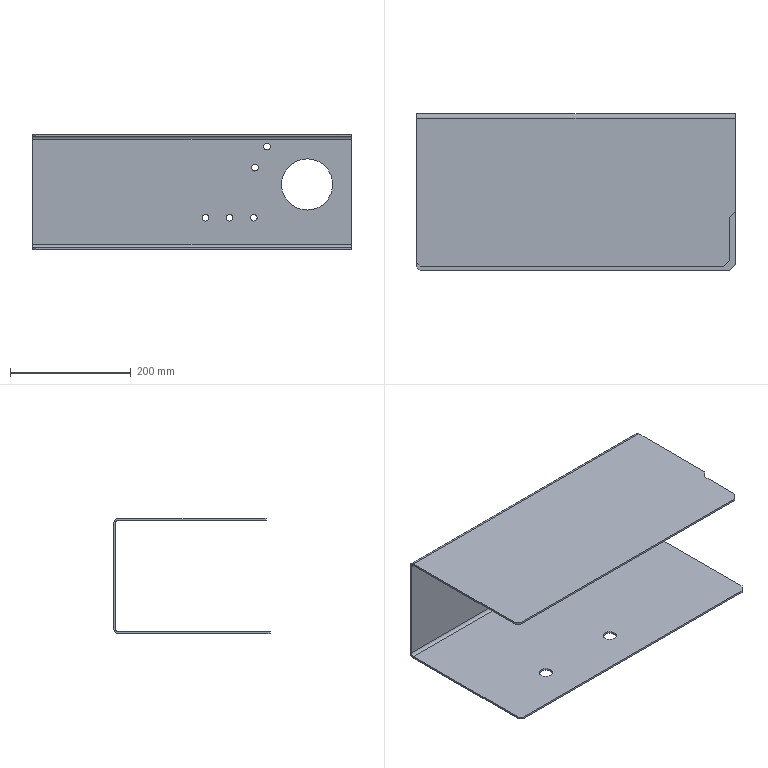Part | SolidWorks | features Chamfer 3, ICE 3, FlatPattern 1, SMBaseFlange 1, SheetMetal 1 | 1 solid | 44 faces | box 529 x 260 x 191.4 mm | volume 1146717 mm3 | plane 24 | cylinder 20 | commonest cylinder face diameters 11 x10 22 x4 10 x2 16.4 x2 85 x2
STEP:
#1=CARTESIAN_POINT('',(123.,68.,-188.2));
#2=VERTEX_POINT('',#1);
#3=CARTESIAN_POINT('',(123.,46.,-188.2));
#4=VERTEX_POINT('',#3);
#5=CARTESIAN_POINT('',(123.,57.,-188.2));
#6=DIRECTION('',(0.,0.,1.));
#7=DIRECTION('',(0.,1.,0.));
#8=AXIS2_PLACEMENT_3D('',#5,#6,#7);
#9=CIRCLE('',#8,11.);
#10=EDGE_CURVE('',#2,#4,#9,.T.);
#11=ORIENTED_EDGE('',*,*,#10,.T.);
#12=CARTESIAN_POINT('',(123.,46.,-191.4));
#13=VERTEX_POINT('',#12);
#14=CARTESIAN_POINT('',(123.,46.,0.001));
#15=DIRECTION('',(0.,0.,-1.));
#16=VECTOR('',#15,1000.);
#17=LINE('',#14,#16);
#18=EDGE_CURVE('',#4,#13,#17,.T.);
#19=ORIENTED_EDGE('',*,*,#18,.T.);
#20=CARTESIAN_POINT('',(123.,68.,-191.4));
#21=VERTEX_POINT('',#20);
#22=CARTESIAN_POINT('',(123.,57.,-191.4));
#23=DIRECTION('',(0.,0.,-1.));
#24=DIRECTION('',(0.,1.,0.));
#25=AXIS2_PLACEMENT_3D('',#22,#23,#24);
#26=CIRCLE('',#25,11.);
#27=EDGE_CURVE('',#13,#21,#26,.T.);
#28=ORIENTED_EDGE('',*,*,#27,.T.);
#29=CARTESIAN_POINT('',(123.,68.,0.001));
#30=DIRECTION('',(0.,0.,-1.));
#31=VECTOR('',#30,1000.);
#32=LINE('',#29,#31);
#33=EDGE_CURVE('',#2,#21,#32,.T.);
#34=ORIENTED_EDGE('',*,*,#33,.F.);
#35=EDGE_LOOP('',(#11,#19,#28,#34));
#36=FACE_OUTER_BOUND('',#35,.T.);
#37=CARTESIAN_POINT('',(123.,57.,0.001));
#38=DIRECTION('',(0.,0.,-1.));
#39=DIRECTION('',(0.,1.,0.));
#40=AXIS2_PLACEMENT_3D('',#37,#38,#39);
#41=CYLINDRICAL_SURFACE('',#40,11.);
#42=ADVANCED_FACE('',(#36),#41,.F.);
#43=CARTESIAN_POINT('',(273.,68.,-188.2));
#44=VERTEX_POINT('',#43);
#45=CARTESIAN_POINT('',(273.,46.,-188.2));
#46=VERTEX_POINT('',#45);
#47=CARTESIAN_POINT('',(273.,57.,-188.2));
#48=DIRECTION('',(0.,0.,1.));
#49=DIRECTION('',(0.,1.,0.));
#50=AXIS2_PLACEMENT_3D('',#47,#48,#49);
#51=CIRCLE('',#50,11.);
#52=EDGE_CURVE('',#44,#46,#51,.T.);
#53=ORIENTED_EDGE('',*,*,#52,.T.);
#54=CARTESIAN_POINT('',(273.,46.,-191.4));
#55=VERTEX_POINT('',#54);
#56=CARTESIAN_POINT('',(273.,46.,0.001));
#57=DIRECTION('',(0.,0.,-1.));
#58=VECTOR('',#57,1000.);
#59=LINE('',#56,#58);
#60=EDGE_CURVE('',#46,#55,#59,.T.);
#61=ORIENTED_EDGE('',*,*,#60,.T.);
#62=CARTESIAN_POINT('',(273.,68.,-191.4));
#63=VERTEX_POINT('',#62);
#64=CARTESIAN_POINT('',(273.,57.,-191.4));
#65=DIRECTION('',(0.,0.,-1.));
#66=DIRECTION('',(0.,1.,0.));
#67=AXIS2_PLACEMENT_3D('',#64,#65,#66);
#68=CIRCLE('',#67,11.);
#69=EDGE_CURVE('',#55,#63,#68,.T.);
#70=ORIENTED_EDGE('',*,*,#69,.T.);
#71=CARTESIAN_POINT('',(273.,68.,0.001));
#72=DIRECTION('',(0.,0.,-1.));
#73=VECTOR('',#72,1000.);
#74=LINE('',#71,#73);
#75=EDGE_CURVE('',#44,#63,#74,.T.);
#76=ORIENTED_EDGE('',*,*,#75,.F.);
#77=EDGE_LOOP('',(#53,#61,#70,#76));
#78=FACE_OUTER_BOUND('',#77,.T.);
#79=CARTESIAN_POINT('',(273.,57.,0.001));
#80=DIRECTION('',(0.,0.,-1.));
#81=DIRECTION('',(0.,1.,0.));
#82=AXIS2_PLACEMENT_3D('',#79,#80,#81);
#83=CYLINDRICAL_SURFACE('',#82,11.);
#84=ADVANCED_FACE('',(#78),#83,.F.);
#85=CARTESIAN_POINT('',(389.,249.8,-14.9));
#86=VERTEX_POINT('',#85);
#87=CARTESIAN_POINT('',(389.,249.8,-25.9));
#88=VERTEX_POINT('',#87);
#89=CARTESIAN_POINT('',(389.,249.8,-20.4));
#90=DIRECTION('',(0.,-1.,0.));
#91=DIRECTION('',(0.,0.,1.));
#92=AXIS2_PLACEMENT_3D('',#89,#90,#91);
#93=CIRCLE('',#92,5.5);
#94=EDGE_CURVE('',#86,#88,#93,.T.);
#95=ORIENTED_EDGE('',*,*,#94,.T.);
#96=CARTESIAN_POINT('',(389.,253.,-25.9));
#97=VERTEX_POINT('',#96);
#98=CARTESIAN_POINT('',(389.,-7.001,-25.9));
#99=DIRECTION('',(0.,1.,0.));
#100=VECTOR('',#99,1000.);
#101=LINE('',#98,#100);
#102=EDGE_CURVE('',#88,#97,#101,.T.);
#103=ORIENTED_EDGE('',*,*,#102,.T.);
#104=CARTESIAN_POINT('',(389.,253.,-14.9));
#105=VERTEX_POINT('',#104);
#106=CARTESIAN_POINT('',(389.,253.,-20.4));
#107=DIRECTION('',(0.,1.,0.));
#108=DIRECTION('',(0.,0.,1.));
#109=AXIS2_PLACEMENT_3D('',#106,#107,#108);
#110=CIRCLE('',#109,5.5);
#111=EDGE_CURVE('',#97,#105,#110,.T.);
#112=ORIENTED_EDGE('',*,*,#111,.T.);
#113=CARTESIAN_POINT('',(389.,-7.001,-14.9));
#114=DIRECTION('',(0.,1.,0.));
#115=VECTOR('',#114,1000.);
#116=LINE('',#113,#115);
#117=EDGE_CURVE('',#86,#105,#116,.T.);
#118=ORIENTED_EDGE('',*,*,#117,.F.);
#119=EDGE_LOOP('',(#95,#103,#112,#118));
#120=FACE_OUTER_BOUND('',#119,.T.);
#121=CARTESIAN_POINT('',(389.,-7.001,-20.4));
#122=DIRECTION('',(0.,1.,0.));
#123=DIRECTION('',(0.,0.,1.));
#124=AXIS2_PLACEMENT_3D('',#121,#122,#123);
#125=CYLINDRICAL_SURFACE('',#124,5.5);
#126=ADVANCED_FACE('',(#120),#125,.F.);
#127=CARTESIAN_POINT('',(367.,249.8,-132.9));
#128=VERTEX_POINT('',#127);
#129=CARTESIAN_POINT('',(367.,249.8,-143.9));
#130=VERTEX_POINT('',#129);
#131=CARTESIAN_POINT('',(367.,249.8,-138.4));
#132=DIRECTION('',(0.,-1.,0.));
#133=DIRECTION('',(0.,0.,1.));
#134=AXIS2_PLACEMENT_3D('',#131,#132,#133);
#135=CIRCLE('',#134,5.5);
#136=EDGE_CURVE('',#128,#130,#135,.T.);
#137=ORIENTED_EDGE('',*,*,#136,.T.);
#138=CARTESIAN_POINT('',(367.,253.,-143.9));
#139=VERTEX_POINT('',#138);
#140=CARTESIAN_POINT('',(367.,-7.001,-143.9));
#141=DIRECTION('',(0.,1.,0.));
#142=VECTOR('',#141,1000.);
#143=LINE('',#140,#142);
#144=EDGE_CURVE('',#130,#139,#143,.T.);
#145=ORIENTED_EDGE('',*,*,#144,.T.);
#146=CARTESIAN_POINT('',(367.,253.,-132.9));
#147=VERTEX_POINT('',#146);
#148=CARTESIAN_POINT('',(367.,253.,-138.4));
#149=DIRECTION('',(0.,1.,0.));
#150=DIRECTION('',(0.,0.,1.));
#151=AXIS2_PLACEMENT_3D('',#148,#149,#150);
#152=CIRCLE('',#151,5.5);
#153=EDGE_CURVE('',#139,#147,#152,.T.);
#154=ORIENTED_EDGE('',*,*,#153,.T.);
#155=CARTESIAN_POINT('',(367.,-7.001,-132.9));
#156=DIRECTION('',(0.,1.,0.));
#157=VECTOR('',#156,1000.);
#158=LINE('',#155,#157);
#159=EDGE_CURVE('',#128,#147,#158,.T.);
#160=ORIENTED_EDGE('',*,*,#159,.F.);
#161=EDGE_LOOP('',(#137,#145,#154,#160));
#162=FACE_OUTER_BOUND('',#161,.T.);
#163=CARTESIAN_POINT('',(367.,-7.001,-138.4));
#164=DIRECTION('',(0.,1.,0.));
#165=DIRECTION('',(0.,0.,1.));
#166=AXIS2_PLACEMENT_3D('',#163,#164,#165);
#167=CYLINDRICAL_SURFACE('',#166,5.5);
#168=ADVANCED_FACE('',(#162),#167,.F.);
#169=CARTESIAN_POINT('',(327.,249.8,-132.9));
#170=VERTEX_POINT('',#169);
#171=CARTESIAN_POINT('',(327.,249.8,-143.9));
#172=VERTEX_POINT('',#171);
#173=CARTESIAN_POINT('',(327.,249.8,-138.4));
#174=DIRECTION('',(0.,-1.,0.));
#175=DIRECTION('',(0.,0.,1.));
#176=AXIS2_PLACEMENT_3D('',#173,#174,#175);
#177=CIRCLE('',#176,5.5);
#178=EDGE_CURVE('',#170,#172,#177,.T.);
#179=ORIENTED_EDGE('',*,*,#178,.T.);
#180=CARTESIAN_POINT('',(327.,253.,-143.9));
#181=VERTEX_POINT('',#180);
#182=CARTESIAN_POINT('',(327.,-7.001,-143.9));
#183=DIRECTION('',(0.,1.,0.));
#184=VECTOR('',#183,1000.);
#185=LINE('',#182,#184);
#186=EDGE_CURVE('',#172,#181,#185,.T.);
#187=ORIENTED_EDGE('',*,*,#186,.T.);
#188=CARTESIAN_POINT('',(327.,253.,-132.9));
#189=VERTEX_POINT('',#188);
#190=CARTESIAN_POINT('',(327.,253.,-138.4));
#191=DIRECTION('',(0.,1.,0.));
#192=DIRECTION('',(0.,0.,1.));
#193=AXIS2_PLACEMENT_3D('',#190,#191,#192);
#194=CIRCLE('',#193,5.5);
#195=EDGE_CURVE('',#181,#189,#194,.T.);
#196=ORIENTED_EDGE('',*,*,#195,.T.);
#197=CARTESIAN_POINT('',(327.,-7.001,-132.9));
#198=DIRECTION('',(0.,1.,0.));
#199=VECTOR('',#198,1000.);
#200=LINE('',#197,#199);
#201=EDGE_CURVE('',#170,#189,#200,.T.);
#202=ORIENTED_EDGE('',*,*,#201,.F.);
#203=EDGE_LOOP('',(#179,#187,#196,#202));
#204=FACE_OUTER_BOUND('',#203,.T.);
#205=CARTESIAN_POINT('',(327.,-7.001,-138.4));
#206=DIRECTION('',(0.,1.,0.));
#207=DIRECTION('',(0.,0.,1.));
#208=AXIS2_PLACEMENT_3D('',#205,#206,#207);
#209=CYLINDRICAL_SURFACE('',#208,5.5);
#210=ADVANCED_FACE('',(#204),#209,.F.);
#211=CARTESIAN_POINT('',(287.,249.8,-132.9));
#212=VERTEX_POINT('',#211);
#213=CARTESIAN_POINT('',(287.,249.8,-143.9));
#214=VERTEX_POINT('',#213);
#215=CARTESIAN_POINT('',(287.,249.8,-138.4));
#216=DIRECTION('',(0.,-1.,0.));
#217=DIRECTION('',(0.,0.,1.));
#218=AXIS2_PLACEMENT_3D('',#215,#216,#217);
#219=CIRCLE('',#218,5.5);
#220=EDGE_CURVE('',#212,#214,#219,.T.);
#221=ORIENTED_EDGE('',*,*,#220,.T.);
#222=CARTESIAN_POINT('',(287.,253.,-143.9));
#223=VERTEX_POINT('',#222);
#224=CARTESIAN_POINT('',(287.,-7.001,-143.9));
#225=DIRECTION('',(0.,1.,0.));
#226=VECTOR('',#225,1000.);
#227=LINE('',#224,#226);
#228=EDGE_CURVE('',#214,#223,#227,.T.);
#229=ORIENTED_EDGE('',*,*,#228,.T.);
#230=CARTESIAN_POINT('',(287.,253.,-132.9));
#231=VERTEX_POINT('',#230);
#232=CARTESIAN_POINT('',(287.,253.,-138.4));
#233=DIRECTION('',(0.,1.,0.));
#234=DIRECTION('',(0.,0.,1.));
#235=AXIS2_PLACEMENT_3D('',#232,#233,#234);
#236=CIRCLE('',#235,5.5);
#237=EDGE_CURVE('',#223,#231,#236,.T.);
#238=ORIENTED_EDGE('',*,*,#237,.T.);
#239=CARTESIAN_POINT('',(287.,-7.001,-132.9));
#240=DIRECTION('',(0.,1.,0.));
#241=VECTOR('',#240,1000.);
#242=LINE('',#239,#241);
#243=EDGE_CURVE('',#212,#231,#242,.T.);
#244=ORIENTED_EDGE('',*,*,#243,.F.);
#245=EDGE_LOOP('',(#221,#229,#238,#244));
#246=FACE_OUTER_BOUND('',#245,.T.);
#247=CARTESIAN_POINT('',(287.,-7.001,-138.4));
#248=DIRECTION('',(0.,1.,0.));
#249=DIRECTION('',(0.,0.,1.));
#250=AXIS2_PLACEMENT_3D('',#247,#248,#249);
#251=CYLINDRICAL_SURFACE('',#250,5.5);
#252=ADVANCED_FACE('',(#246),#251,.F.);
#253=CARTESIAN_POINT('',(369.,249.8,-49.9));
#254=VERTEX_POINT('',#253);
#255=CARTESIAN_POINT('',(369.,249.8,-60.9));
#256=VERTEX_POINT('',#255);
#257=CARTESIAN_POINT('',(369.,249.8,-55.4));
#258=DIRECTION('',(0.,-1.,0.));
#259=DIRECTION('',(0.,0.,1.));
#260=AXIS2_PLACEMENT_3D('',#257,#258,#259);
#261=CIRCLE('',#260,5.5);
#262=EDGE_CURVE('',#254,#256,#261,.T.);
#263=ORIENTED_EDGE('',*,*,#262,.T.);
#264=CARTESIAN_POINT('',(369.,253.,-60.9));
#265=VERTEX_POINT('',#264);
#266=CARTESIAN_POINT('',(369.,-7.001,-60.9));
#267=DIRECTION('',(0.,1.,0.));
#268=VECTOR('',#267,1000.);
#269=LINE('',#266,#268);
#270=EDGE_CURVE('',#256,#265,#269,.T.);
#271=ORIENTED_EDGE('',*,*,#270,.T.);
#272=CARTESIAN_POINT('',(369.,253.,-49.9));
#273=VERTEX_POINT('',#272);
#274=CARTESIAN_POINT('',(369.,253.,-55.4));
#275=DIRECTION('',(0.,1.,0.));
#276=DIRECTION('',(0.,0.,1.));
#277=AXIS2_PLACEMENT_3D('',#274,#275,#276);
#278=CIRCLE('',#277,5.5);
#279=EDGE_CURVE('',#265,#273,#278,.T.);
#280=ORIENTED_EDGE('',*,*,#279,.T.);
#281=CARTESIAN_POINT('',(369.,-7.001,-49.9));
#282=DIRECTION('',(0.,1.,0.));
#283=VECTOR('',#282,1000.);
#284=LINE('',#281,#283);
#285=EDGE_CURVE('',#254,#273,#284,.T.);
#286=ORIENTED_EDGE('',*,*,#285,.F.);
#287=EDGE_LOOP('',(#263,#271,#280,#286));
#288=FACE_OUTER_BOUND('',#287,.T.);
#289=CARTESIAN_POINT('',(369.,-7.001,-55.4));
#290=DIRECTION('',(0.,1.,0.));
#291=DIRECTION('',(0.,0.,1.));
#292=AXIS2_PLACEMENT_3D('',#289,#290,#291);
#293=CYLINDRICAL_SURFACE('',#292,5.5);
#294=ADVANCED_FACE('',(#288),#293,.F.);
#295=CARTESIAN_POINT('',(455.5,249.8,-40.7));
#296=VERTEX_POINT('',#295);
#297=CARTESIAN_POINT('',(455.5,249.8,-125.7));
#298=VERTEX_POINT('',#297);
#299=CARTESIAN_POINT('',(455.5,249.8,-83.2));
#300=DIRECTION('',(0.,-1.,0.));
#301=DIRECTION('',(0.,0.,1.));
#302=AXIS2_PLACEMENT_3D('',#299,#300,#301);
#303=CIRCLE('',#302,42.5);
#304=EDGE_CURVE('',#296,#298,#303,.T.);
#305=ORIENTED_EDGE('',*,*,#304,.T.);
#306=CARTESIAN_POINT('',(455.5,253.,-125.7));
#307=VERTEX_POINT('',#306);
#308=CARTESIAN_POINT('',(455.5,-7.001,-125.7));
#309=DIRECTION('',(0.,1.,0.));
#310=VECTOR('',#309,1000.);
#311=LINE('',#308,#310);
#312=EDGE_CURVE('',#298,#307,#311,.T.);
#313=ORIENTED_EDGE('',*,*,#312,.T.);
#314=CARTESIAN_POINT('',(455.5,253.,-40.7));
#315=VERTEX_POINT('',#314);
#316=CARTESIAN_POINT('',(455.5,253.,-83.2));
#317=DIRECTION('',(0.,1.,0.));
#318=DIRECTION('',(0.,0.,1.));
#319=AXIS2_PLACEMENT_3D('',#316,#317,#318);
#320=CIRCLE('',#319,42.5);
#321=EDGE_CURVE('',#307,#315,#320,.T.);
#322=ORIENTED_EDGE('',*,*,#321,.T.);
#323=CARTESIAN_POINT('',(455.5,-7.001,-40.7));
#324=DIRECTION('',(0.,1.,0.));
#325=VECTOR('',#324,1000.);
#326=LINE('',#323,#325);
#327=EDGE_CURVE('',#296,#315,#326,.T.);
#328=ORIENTED_EDGE('',*,*,#327,.F.);
#329=EDGE_LOOP('',(#305,#313,#322,#328));
#330=FACE_OUTER_BOUND('',#329,.T.);
#331=CARTESIAN_POINT('',(455.5,-7.001,-83.2));
#332=DIRECTION('',(0.,1.,0.));
#333=DIRECTION('',(0.,0.,1.));
#334=AXIS2_PLACEMENT_3D('',#331,#332,#333);
#335=CYLINDRICAL_SURFACE('',#334,42.5);
#336=ADVANCED_FACE('',(#330),#335,.F.);
#337=CARTESIAN_POINT('',(509.,0.,0.));
#338=VERTEX_POINT('',#337);
#339=CARTESIAN_POINT('',(6.,0.,0.));
#340=VERTEX_POINT('',#339);
#341=CARTESIAN_POINT('',(529.,0.,0.));
#342=DIRECTION('',(-1.,0.,0.));
#343=VECTOR('',#342,1000.);
#344=LINE('',#341,#343);
#345=EDGE_CURVE('',#338,#340,#344,.T.);
#346=ORIENTED_EDGE('',*,*,#345,.F.);
#347=CARTESIAN_POINT('',(519.,10.,0.));
#348=VERTEX_POINT('',#347);
#349=CARTESIAN_POINT('',(519.,10.,0.));
#350=DIRECTION('',(0.7071,0.7071,0.));
#351=VECTOR('',#350,1000.);
#352=LINE('',#349,#351);
#353=EDGE_CURVE('',#338,#348,#352,.T.);
#354=ORIENTED_EDGE('',*,*,#353,.T.);
#355=CARTESIAN_POINT('',(519.,80.,0.));
#356=VERTEX_POINT('',#355);
#357=CARTESIAN_POINT('',(519.,0.,0.));
#358=DIRECTION('',(0.,1.,0.));
#359=VECTOR('',#358,1000.);
#360=LINE('',#357,#359);
#361=EDGE_CURVE('',#348,#356,#360,.T.);
#362=ORIENTED_EDGE('',*,*,#361,.T.);
#363=CARTESIAN_POINT('',(529.,90.,0.));
#364=VERTEX_POINT('',#363);
#365=CARTESIAN_POINT('',(519.,80.,0.));
#366=DIRECTION('',(0.7071,0.7071,0.));
#367=VECTOR('',#366,1000.);
#368=LINE('',#365,#367);
#369=EDGE_CURVE('',#356,#364,#368,.T.);
#370=ORIENTED_EDGE('',*,*,#369,.T.);
#371=CARTESIAN_POINT('',(529.,244.8,0.));
#372=VERTEX_POINT('',#371);
#373=CARTESIAN_POINT('',(529.,0.,0.));
#374=DIRECTION('',(0.,1.,0.));
#375=VECTOR('',#374,1000.);
#376=LINE('',#373,#375);
#377=EDGE_CURVE('',#364,#372,#376,.T.);
#378=ORIENTED_EDGE('',*,*,#377,.T.);
#379=CARTESIAN_POINT('',(0.,244.8,0.));
#380=VERTEX_POINT('',#379);
#381=CARTESIAN_POINT('',(529.,244.8,0.));
#382=DIRECTION('',(-1.,0.,0.));
#383=VECTOR('',#382,1000.);
#384=LINE('',#381,#383);
#385=EDGE_CURVE('',#372,#380,#384,.T.);
#386=ORIENTED_EDGE('',*,*,#385,.T.);
#387=CARTESIAN_POINT('',(0.,6.,0.));
#388=VERTEX_POINT('',#387);
#389=CARTESIAN_POINT('',(0.,0.,0.));
#390=DIRECTION('',(0.,1.,0.));
#391=VECTOR('',#390,1000.);
#392=LINE('',#389,#391);
#393=EDGE_CURVE('',#388,#380,#392,.T.);
#394=ORIENTED_EDGE('',*,*,#393,.F.);
#395=CARTESIAN_POINT('',(267.5,-261.5,0.));
#396=DIRECTION('',(0.7071,-0.7071,0.));
#397=VECTOR('',#396,1000.);
#398=LINE('',#395,#397);
#399=EDGE_CURVE('',#388,#340,#398,.T.);
#400=ORIENTED_EDGE('',*,*,#399,.T.);
#401=EDGE_LOOP('',(#346,#354,#362,#370,#378,#386,#394,#400));
#402=FACE_OUTER_BOUND('',#401,.T.);
#403=CARTESIAN_POINT('',(529.,0.,0.));
#404=DIRECTION('',(0.,0.,1.));
#405=DIRECTION('',(1.,0.,0.));
#406=AXIS2_PLACEMENT_3D('',#403,#404,#405);
#407=PLANE('',#406);
#408=ADVANCED_FACE('',(#402),#407,.T.);
#409=CARTESIAN_POINT('',(509.,0.,-3.2));
#410=VERTEX_POINT('',#409);
#411=CARTESIAN_POINT('',(6.,0.,-3.2));
#412=VERTEX_POINT('',#411);
#413=CARTESIAN_POINT('',(529.,0.,-3.2));
#414=DIRECTION('',(-1.,0.,0.));
#415=VECTOR('',#414,1000.);
#416=LINE('',#413,#415);
#417=EDGE_CURVE('',#410,#412,#416,.T.);
#418=ORIENTED_EDGE('',*,*,#417,.F.);
#419=CARTESIAN_POINT('',(509.,0.,-3.2));
#420=DIRECTION('',(0.,0.,1.));
#421=VECTOR('',#420,1000.);
#422=LINE('',#419,#421);
#423=EDGE_CURVE('',#410,#338,#422,.T.);
#424=ORIENTED_EDGE('',*,*,#423,.T.);
#425=ORIENTED_EDGE('',*,*,#345,.T.);
#426=CARTESIAN_POINT('',(6.,0.,-3.2));
#427=DIRECTION('',(0.,0.,-1.));
#428=VECTOR('',#427,1000.);
#429=LINE('',#426,#428);
#430=EDGE_CURVE('',#340,#412,#429,.T.);
#431=ORIENTED_EDGE('',*,*,#430,.T.);
#432=EDGE_LOOP('',(#418,#424,#425,#431));
#433=FACE_OUTER_BOUND('',#432,.T.);
#434=CARTESIAN_POINT('',(529.,0.,-3.2));
#435=DIRECTION('',(0.,-1.,0.));
#436=DIRECTION('',(0.,0.,-1.));
#437=AXIS2_PLACEMENT_3D('',#434,#435,#436);
#438=PLANE('',#437);
#439=ADVANCED_FACE('',(#433),#438,.T.);
#440=CARTESIAN_POINT('',(519.,10.,-3.2));
#441=VERTEX_POINT('',#440);
#442=CARTESIAN_POINT('',(519.,80.,-3.2));
#443=VERTEX_POINT('',#442);
#444=CARTESIAN_POINT('',(519.,0.,-3.2));
#445=DIRECTION('',(0.,1.,0.));
#446=VECTOR('',#445,1000.);
#447=LINE('',#444,#446);
#448=EDGE_CURVE('',#441,#443,#447,.T.);
#449=ORIENTED_EDGE('',*,*,#448,.F.);
#450=CARTESIAN_POINT('',(509.,0.,-3.2));
#451=DIRECTION('',(-0.7071,-0.7071,0.));
#452=VECTOR('',#451,1000.);
#453=LINE('',#450,#452);
#454=EDGE_CURVE('',#441,#410,#453,.T.);
#455=ORIENTED_EDGE('',*,*,#454,.T.);
#456=ORIENTED_EDGE('',*,*,#417,.T.);
#457=CARTESIAN_POINT('',(0.,6.,-3.2));
#458=VERTEX_POINT('',#457);
#459=CARTESIAN_POINT('',(0.,6.,-3.2));
#460=DIRECTION('',(-0.7071,0.7071,0.));
#461=VECTOR('',#460,1000.);
#462=LINE('',#459,#461);
#463=EDGE_CURVE('',#412,#458,#462,.T.);
#464=ORIENTED_EDGE('',*,*,#463,.T.);
#465=CARTESIAN_POINT('',(0.,244.8,-3.2));
#466=VERTEX_POINT('',#465);
#467=CARTESIAN_POINT('',(0.,0.,-3.2));
#468=DIRECTION('',(0.,1.,0.));
#469=VECTOR('',#468,1000.);
#470=LINE('',#467,#469);
#471=EDGE_CURVE('',#458,#466,#470,.T.);
#472=ORIENTED_EDGE('',*,*,#471,.T.);
#473=CARTESIAN_POINT('',(529.,244.8,-3.2));
#474=VERTEX_POINT('',#473);
#475=CARTESIAN_POINT('',(529.,244.8,-3.2));
#476=DIRECTION('',(-1.,0.,0.));
#477=VECTOR('',#476,1000.);
#478=LINE('',#475,#477);
#479=EDGE_CURVE('',#474,#466,#478,.T.);
#480=ORIENTED_EDGE('',*,*,#479,.F.);
#481=CARTESIAN_POINT('',(529.,90.,-3.2));
#482=VERTEX_POINT('',#481);
#483=CARTESIAN_POINT('',(529.,0.,-3.2));
#484=DIRECTION('',(0.,1.,0.));
#485=VECTOR('',#484,1000.);
#486=LINE('',#483,#485);
#487=EDGE_CURVE('',#482,#474,#486,.T.);
#488=ORIENTED_EDGE('',*,*,#487,.F.);
#489=CARTESIAN_POINT('',(519.,80.,-3.2));
#490=DIRECTION('',(0.7071,0.7071,0.));
#491=VECTOR('',#490,1000.);
#492=LINE('',#489,#491);
#493=EDGE_CURVE('',#443,#482,#492,.T.);
#494=ORIENTED_EDGE('',*,*,#493,.F.);
#495=EDGE_LOOP('',(#449,#455,#456,#464,#472,#480,#488,#494));
#496=FACE_OUTER_BOUND('',#495,.T.);
#497=CARTESIAN_POINT('',(529.,0.,-3.2));
#498=DIRECTION('',(0.,0.,1.));
#499=DIRECTION('',(1.,0.,0.));
#500=AXIS2_PLACEMENT_3D('',#497,#498,#499);
#501=PLANE('',#500);
#502=ADVANCED_FACE('',(#496),#501,.F.);
#503=ORIENTED_EDGE('',*,*,#377,.F.);
#504=CARTESIAN_POINT('',(529.,90.,-3.2));
#505=DIRECTION('',(0.,0.,1.));
#506=VECTOR('',#505,1000.);
#507=LINE('',#504,#506);
#508=EDGE_CURVE('',#482,#364,#507,.T.);
#509=ORIENTED_EDGE('',*,*,#508,.F.);
#510=ORIENTED_EDGE('',*,*,#487,.T.);
#511=CARTESIAN_POINT('',(529.,244.8,-3.2));
#512=DIRECTION('',(0.,0.,1.));
#513=VECTOR('',#512,1000.);
#514=LINE('',#511,#513);
#515=EDGE_CURVE('',#474,#372,#514,.T.);
#516=ORIENTED_EDGE('',*,*,#515,.T.);
#517=EDGE_LOOP('',(#503,#509,#510,#516));
#518=FACE_OUTER_BOUND('',#517,.T.);
#519=CARTESIAN_POINT('',(529.,244.8,-183.2));
#520=DIRECTION('',(1.,0.,0.));
#521=DIRECTION('',(0.,0.,-1.));
#522=AXIS2_PLACEMENT_3D('',#519,#520,#521);
#523=PLANE('',#522);
#524=ADVANCED_FACE('',(#518),#523,.T.);
#525=CARTESIAN_POINT('',(529.,253.,-8.2));
#526=VERTEX_POINT('',#525);
#527=CARTESIAN_POINT('',(529.,249.8,-8.2));
#528=VERTEX_POINT('',#527);
#529=CARTESIAN_POINT('',(529.,253.,-8.2));
#530=DIRECTION('',(0.,-1.,0.));
#531=VECTOR('',#530,1000.);
#532=LINE('',#529,#531);
#533=EDGE_CURVE('',#526,#528,#532,.T.);
#534=ORIENTED_EDGE('',*,*,#533,.F.);
#535=CARTESIAN_POINT('',(529.,244.8,-8.2));
#536=DIRECTION('',(-1.,0.,0.));
#537=DIRECTION('',(0.,0.,-1.));
#538=AXIS2_PLACEMENT_3D('',#535,#536,#537);
#539=CIRCLE('',#538,8.2);
#540=EDGE_CURVE('',#372,#526,#539,.T.);
#541=ORIENTED_EDGE('',*,*,#540,.F.);
#542=ORIENTED_EDGE('',*,*,#515,.F.);
#543=CARTESIAN_POINT('',(529.,244.8,-8.2));
#544=DIRECTION('',(-1.,0.,0.));
#545=DIRECTION('',(0.,0.,-1.));
#546=AXIS2_PLACEMENT_3D('',#543,#544,#545);
#547=CIRCLE('',#546,5.);
#548=EDGE_CURVE('',#474,#528,#547,.T.);
#549=ORIENTED_EDGE('',*,*,#548,.T.);
#550=EDGE_LOOP('',(#534,#541,#542,#549));
#551=FACE_OUTER_BOUND('',#550,.T.);
#552=CARTESIAN_POINT('',(529.,253.,-8.2));
#553=DIRECTION('',(1.,0.,0.));
#554=DIRECTION('',(0.,0.,-1.));
#555=AXIS2_PLACEMENT_3D('',#552,#553,#554);
#556=PLANE('',#555);
#557=ADVANCED_FACE('',(#551),#556,.T.);
#558=CARTESIAN_POINT('',(529.,253.,-183.2));
#559=VERTEX_POINT('',#558);
#560=CARTESIAN_POINT('',(529.,253.,0.));
#561=DIRECTION('',(0.,0.,-1.));
#562=VECTOR('',#561,1000.);
#563=LINE('',#560,#562);
#564=EDGE_CURVE('',#526,#559,#563,.T.);
#565=ORIENTED_EDGE('',*,*,#564,.F.);
#566=ORIENTED_EDGE('',*,*,#533,.T.);
#567=CARTESIAN_POINT('',(529.,249.8,-183.2));
#568=VERTEX_POINT('',#567);
#569=CARTESIAN_POINT('',(529.,249.8,0.));
#570=DIRECTION('',(0.,0.,-1.));
#571=VECTOR('',#570,1000.);
#572=LINE('',#569,#571);
#573=EDGE_CURVE('',#528,#568,#572,.T.);
#574=ORIENTED_EDGE('',*,*,#573,.T.);
#575=CARTESIAN_POINT('',(529.,249.8,-183.2));
#576=DIRECTION('',(0.,1.,0.));
#577=VECTOR('',#576,1000.);
#578=LINE('',#575,#577);
#579=EDGE_CURVE('',#568,#559,#578,.T.);
#580=ORIENTED_EDGE('',*,*,#579,.T.);
#581=EDGE_LOOP('',(#565,#566,#574,#580));
#582=FACE_OUTER_BOUND('',#581,.T.);
#583=CARTESIAN_POINT('',(529.,244.8,-3.2));
#584=DIRECTION('',(1.,0.,0.));
#585=DIRECTION('',(0.,0.,-1.));
#586=AXIS2_PLACEMENT_3D('',#583,#584,#585);
#587=PLANE('',#586);
#588=ADVANCED_FACE('',(#582),#587,.T.);
#589=CARTESIAN_POINT('',(0.,244.8,0.));
#590=DIRECTION('',(0.,0.,-1.));
#591=VECTOR('',#590,1000.);
#592=LINE('',#589,#591);
#593=EDGE_CURVE('',#380,#466,#592,.T.);
#594=ORIENTED_EDGE('',*,*,#593,.F.);
#595=CARTESIAN_POINT('',(0.,253.,-8.2));
#596=VERTEX_POINT('',#595);
#597=CARTESIAN_POINT('',(0.,244.8,-8.2));
#598=DIRECTION('',(-1.,0.,0.));
#599=DIRECTION('',(0.,0.,-1.));
#600=AXIS2_PLACEMENT_3D('',#597,#598,#599);
#601=CIRCLE('',#600,8.2);
#602=EDGE_CURVE('',#380,#596,#601,.T.);
#603=ORIENTED_EDGE('',*,*,#602,.T.);
#604=CARTESIAN_POINT('',(0.,249.8,-8.2));
#605=VERTEX_POINT('',#604);
#606=CARTESIAN_POINT('',(0.,249.8,-8.2));
#607=DIRECTION('',(0.,1.,0.));
#608=VECTOR('',#607,1000.);
#609=LINE('',#606,#608);
#610=EDGE_CURVE('',#605,#596,#609,.T.);
#611=ORIENTED_EDGE('',*,*,#610,.F.);
#612=CARTESIAN_POINT('',(0.,244.8,-8.2));
#613=DIRECTION('',(-1.,0.,0.));
#614=DIRECTION('',(0.,0.,-1.));
#615=AXIS2_PLACEMENT_3D('',#612,#613,#614);
#616=CIRCLE('',#615,5.);
#617=EDGE_CURVE('',#466,#605,#616,.T.);
#618=ORIENTED_EDGE('',*,*,#617,.F.);
#619=EDGE_LOOP('',(#594,#603,#611,#618));
#620=FACE_OUTER_BOUND('',#619,.T.);
#621=CARTESIAN_POINT('',(0.,244.8,0.));
#622=DIRECTION('',(-1.,0.,0.));
#623=DIRECTION('',(0.,0.,1.));
#624=AXIS2_PLACEMENT_3D('',#621,#622,#623);
#625=PLANE('',#624);
#626=ADVANCED_FACE('',(#620),#625,.T.);
#627=ORIENTED_EDGE('',*,*,#471,.F.);
#628=CARTESIAN_POINT('',(0.,6.,-8.2));
#629=DIRECTION('',(0.,0.,1.));
#630=VECTOR('',#629,1000.);
#631=LINE('',#628,#630);
#632=EDGE_CURVE('',#458,#388,#631,.T.);
#633=ORIENTED_EDGE('',*,*,#632,.T.);
#634=ORIENTED_EDGE('',*,*,#393,.T.);
#635=ORIENTED_EDGE('',*,*,#593,.T.);
#636=EDGE_LOOP('',(#627,#633,#634,#635));
#637=FACE_OUTER_BOUND('',#636,.T.);
#638=CARTESIAN_POINT('',(0.,249.8,-8.2));
#639=DIRECTION('',(-1.,0.,0.));
#640=DIRECTION('',(0.,0.,1.));
#641=AXIS2_PLACEMENT_3D('',#638,#639,#640);
#642=PLANE('',#641);
#643=ADVANCED_FACE('',(#637),#642,.T.);
#644=CARTESIAN_POINT('',(529.,244.8,-191.4));
#645=VERTEX_POINT('',#644);
#646=CARTESIAN_POINT('',(529.,244.8,-188.2));
#647=VERTEX_POINT('',#646);
#648=CARTESIAN_POINT('',(529.,244.8,-191.4));
#649=DIRECTION('',(0.,0.,1.));
#650=VECTOR('',#649,1000.);
#651=LINE('',#648,#650);
#652=EDGE_CURVE('',#645,#647,#651,.T.);
#653=ORIENTED_EDGE('',*,*,#652,.F.);
#654=CARTESIAN_POINT('',(529.,244.8,-183.2));
#655=DIRECTION('',(-1.,0.,0.));
#656=DIRECTION('',(0.,0.,-1.));
#657=AXIS2_PLACEMENT_3D('',#654,#655,#656);
#658=CIRCLE('',#657,8.2);
#659=EDGE_CURVE('',#559,#645,#658,.T.);
#660=ORIENTED_EDGE('',*,*,#659,.F.);
#661=ORIENTED_EDGE('',*,*,#579,.F.);
#662=CARTESIAN_POINT('',(529.,244.8,-183.2));
#663=DIRECTION('',(-1.,0.,0.));
#664=DIRECTION('',(0.,0.,-1.));
#665=AXIS2_PLACEMENT_3D('',#662,#663,#664);
#666=CIRCLE('',#665,5.);
#667=EDGE_CURVE('',#568,#647,#666,.T.);
#668=ORIENTED_EDGE('',*,*,#667,.T.);
#669=EDGE_LOOP('',(#653,#660,#661,#668));
#670=FACE_OUTER_BOUND('',#669,.T.);
#671=CARTESIAN_POINT('',(529.,244.8,-191.4));
#672=DIRECTION('',(1.,0.,0.));
#673=DIRECTION('',(0.,0.,-1.));
#674=AXIS2_PLACEMENT_3D('',#671,#672,#673);
#675=PLANE('',#674);
#676=ADVANCED_FACE('',(#670),#675,.T.);
#677=CARTESIAN_POINT('',(529.,3.,-188.2));
#678=VERTEX_POINT('',#677);
#679=CARTESIAN_POINT('',(529.,253.,-188.2));
#680=DIRECTION('',(0.,-1.,0.));
#681=VECTOR('',#680,1000.);
#682=LINE('',#679,#681);
#683=EDGE_CURVE('',#647,#678,#682,.T.);
#684=ORIENTED_EDGE('',*,*,#683,.T.);
#685=CARTESIAN_POINT('',(529.,3.,-191.4));
#686=VERTEX_POINT('',#685);
#687=CARTESIAN_POINT('',(529.,3.,-183.2));
#688=DIRECTION('',(0.,0.,-1.));
#689=VECTOR('',#688,1000.);
#690=LINE('',#687,#689);
#691=EDGE_CURVE('',#678,#686,#690,.T.);
#692=ORIENTED_EDGE('',*,*,#691,.T.);
#693=CARTESIAN_POINT('',(529.,253.,-191.4));
#694=DIRECTION('',(0.,-1.,0.));
#695=VECTOR('',#694,1000.);
#696=LINE('',#693,#695);
#697=EDGE_CURVE('',#645,#686,#696,.T.);
#698=ORIENTED_EDGE('',*,*,#697,.F.);
#699=ORIENTED_EDGE('',*,*,#652,.T.);
#700=EDGE_LOOP('',(#684,#692,#698,#699));
#701=FACE_OUTER_BOUND('',#700,.T.);
#702=CARTESIAN_POINT('',(529.,249.8,-183.2));
#703=DIRECTION('',(1.,0.,0.));
#704=DIRECTION('',(0.,0.,-1.));
#705=AXIS2_PLACEMENT_3D('',#702,#703,#704);
#706=PLANE('',#705);
#707=ADVANCED_FACE('',(#701),#706,.T.);
#708=CARTESIAN_POINT('',(0.,253.,-183.2));
#709=VERTEX_POINT('',#708);
#710=CARTESIAN_POINT('',(0.,249.8,-183.2));
#711=VERTEX_POINT('',#710);
#712=CARTESIAN_POINT('',(0.,253.,-183.2));
#713=DIRECTION('',(0.,-1.,0.));
#714=VECTOR('',#713,1000.);
#715=LINE('',#712,#714);
#716=EDGE_CURVE('',#709,#711,#715,.T.);
#717=ORIENTED_EDGE('',*,*,#716,.F.);
#718=CARTESIAN_POINT('',(0.,244.8,-191.4));
#719=VERTEX_POINT('',#718);
#720=CARTESIAN_POINT('',(0.,244.8,-183.2));
#721=DIRECTION('',(-1.,0.,0.));
#722=DIRECTION('',(0.,0.,-1.));
#723=AXIS2_PLACEMENT_3D('',#720,#721,#722);
#724=CIRCLE('',#723,8.2);
#725=EDGE_CURVE('',#709,#719,#724,.T.);
#726=ORIENTED_EDGE('',*,*,#725,.T.);
#727=CARTESIAN_POINT('',(0.,244.8,-188.2));
#728=VERTEX_POINT('',#727);
#729=CARTESIAN_POINT('',(0.,244.8,-188.2));
#730=DIRECTION('',(0.,0.,-1.));
#731=VECTOR('',#730,1000.);
#732=LINE('',#729,#731);
#733=EDGE_CURVE('',#728,#719,#732,.T.);
#734=ORIENTED_EDGE('',*,*,#733,.F.);
#735=CARTESIAN_POINT('',(0.,244.8,-183.2));
#736=DIRECTION('',(-1.,0.,0.));
#737=DIRECTION('',(0.,0.,-1.));
#738=AXIS2_PLACEMENT_3D('',#735,#736,#737);
#739=CIRCLE('',#738,5.);
#740=EDGE_CURVE('',#711,#728,#739,.T.);
#741=ORIENTED_EDGE('',*,*,#740,.F.);
#742=EDGE_LOOP('',(#717,#726,#734,#741));
#743=FACE_OUTER_BOUND('',#742,.T.);
#744=CARTESIAN_POINT('',(0.,253.,-183.2));
#745=DIRECTION('',(-1.,0.,0.));
#746=DIRECTION('',(0.,0.,1.));
#747=AXIS2_PLACEMENT_3D('',#744,#745,#746);
#748=PLANE('',#747);
#749=ADVANCED_FACE('',(#743),#748,.T.);
#750=CARTESIAN_POINT('',(0.,253.,0.));
#751=DIRECTION('',(0.,0.,-1.));
#752=VECTOR('',#751,1000.);
#753=LINE('',#750,#752);
#754=EDGE_CURVE('',#596,#709,#753,.T.);
#755=ORIENTED_EDGE('',*,*,#754,.T.);
#756=ORIENTED_EDGE('',*,*,#716,.T.);
#757=CARTESIAN_POINT('',(0.,249.8,0.));
#758=DIRECTION('',(0.,0.,-1.));
#759=VECTOR('',#758,1000.);
#760=LINE('',#757,#759);
#761=EDGE_CURVE('',#605,#711,#760,.T.);
#762=ORIENTED_EDGE('',*,*,#761,.F.);
#763=ORIENTED_EDGE('',*,*,#610,.T.);
#764=EDGE_LOOP('',(#755,#756,#762,#763));
#765=FACE_OUTER_BOUND('',#764,.T.);
#766=CARTESIAN_POINT('',(0.,244.8,-188.2));
#767=DIRECTION('',(-1.,0.,0.));
#768=DIRECTION('',(0.,0.,1.));
#769=AXIS2_PLACEMENT_3D('',#766,#767,#768);
#770=PLANE('',#769);
#771=ADVANCED_FACE('',(#765),#770,.T.);
#772=ORIENTED_EDGE('',*,*,#10,.F.);
#773=CARTESIAN_POINT('',(123.,57.,-188.2));
#774=DIRECTION('',(0.,0.,1.));
#775=DIRECTION('',(0.,1.,0.));
#776=AXIS2_PLACEMENT_3D('',#773,#774,#775);
#777=CIRCLE('',#776,11.);
#778=EDGE_CURVE('',#4,#2,#777,.T.);
#779=ORIENTED_EDGE('',*,*,#778,.F.);
#780=EDGE_LOOP('',(#772,#779));
#781=FACE_BOUND('',#780,.T.);
#782=ORIENTED_EDGE('',*,*,#52,.F.);
#783=CARTESIAN_POINT('',(273.,57.,-188.2));
#784=DIRECTION('',(0.,0.,1.));
#785=DIRECTION('',(0.,1.,0.));
#786=AXIS2_PLACEMENT_3D('',#783,#784,#785);
#787=CIRCLE('',#786,11.);
#788=EDGE_CURVE('',#46,#44,#787,.T.);
#789=ORIENTED_EDGE('',*,*,#788,.F.);
#790=EDGE_LOOP('',(#782,#789));
#791=FACE_BOUND('',#790,.T.);
#792=CARTESIAN_POINT('',(519.,-7.,-188.2));
#793=VERTEX_POINT('',#792);
#794=CARTESIAN_POINT('',(6.,-7.,-188.2));
#795=VERTEX_POINT('',#794);
#796=CARTESIAN_POINT('',(529.,-7.,-188.2));
#797=DIRECTION('',(-1.,0.,0.));
#798=VECTOR('',#797,1000.);
#799=LINE('',#796,#798);
#800=EDGE_CURVE('',#793,#795,#799,.T.);
#801=ORIENTED_EDGE('',*,*,#800,.F.);
#802=CARTESIAN_POINT('',(519.,-7.,-188.2));
#803=DIRECTION('',(0.7071,0.7071,0.));
#804=VECTOR('',#803,1000.);
#805=LINE('',#802,#804);
#806=EDGE_CURVE('',#793,#678,#805,.T.);
#807=ORIENTED_EDGE('',*,*,#806,.T.);
#808=ORIENTED_EDGE('',*,*,#683,.F.);
#809=CARTESIAN_POINT('',(529.,244.8,-188.2));
#810=DIRECTION('',(-1.,0.,0.));
#811=VECTOR('',#810,1000.);
#812=LINE('',#809,#811);
#813=EDGE_CURVE('',#647,#728,#812,.T.);
#814=ORIENTED_EDGE('',*,*,#813,.T.);
#815=CARTESIAN_POINT('',(0.,-1.,-188.2));
#816=VERTEX_POINT('',#815);
#817=CARTESIAN_POINT('',(0.,253.,-188.2));
#818=DIRECTION('',(0.,-1.,0.));
#819=VECTOR('',#818,1000.);
#820=LINE('',#817,#819);
#821=EDGE_CURVE('',#728,#816,#820,.T.);
#822=ORIENTED_EDGE('',*,*,#821,.T.);
#823=CARTESIAN_POINT('',(0.,-1.,-188.2));
#824=DIRECTION('',(0.7071,-0.7071,0.));
#825=VECTOR('',#824,1000.);
#826=LINE('',#823,#825);
#827=EDGE_CURVE('',#816,#795,#826,.T.);
#828=ORIENTED_EDGE('',*,*,#827,.T.);
#829=EDGE_LOOP('',(#801,#807,#808,#814,#822,#828));
#830=FACE_OUTER_BOUND('',#829,.T.);
#831=CARTESIAN_POINT('',(529.,253.,-188.2));
#832=DIRECTION('',(0.,0.,-1.));
#833=DIRECTION('',(0.,1.,0.));
#834=AXIS2_PLACEMENT_3D('',#831,#832,#833);
#835=PLANE('',#834);
#836=ADVANCED_FACE('',(#781,#791,#830),#835,.F.);
#837=CARTESIAN_POINT('',(519.,-7.,-191.4));
#838=VERTEX_POINT('',#837);
#839=CARTESIAN_POINT('',(6.,-7.,-191.4));
#840=VERTEX_POINT('',#839);
#841=CARTESIAN_POINT('',(529.,-7.,-191.4));
#842=DIRECTION('',(-1.,0.,0.));
#843=VECTOR('',#842,1000.);
#844=LINE('',#841,#843);
#845=EDGE_CURVE('',#838,#840,#844,.T.);
#846=ORIENTED_EDGE('',*,*,#845,.F.);
#847=CARTESIAN_POINT('',(519.,-7.,-191.4));
#848=DIRECTION('',(0.,0.,1.));
#849=VECTOR('',#848,1000.);
#850=LINE('',#847,#849);
#851=EDGE_CURVE('',#838,#793,#850,.T.);
#852=ORIENTED_EDGE('',*,*,#851,.T.);
#853=ORIENTED_EDGE('',*,*,#800,.T.);
#854=CARTESIAN_POINT('',(6.,-7.,-191.4));
#855=DIRECTION('',(0.,0.,-1.));
#856=VECTOR('',#855,1000.);
#857=LINE('',#854,#856);
#858=EDGE_CURVE('',#795,#840,#857,.T.);
#859=ORIENTED_EDGE('',*,*,#858,.T.);
#860=EDGE_LOOP('',(#846,#852,#853,#859));
#861=FACE_OUTER_BOUND('',#860,.T.);
#862=CARTESIAN_POINT('',(529.,-7.,-191.4));
#863=DIRECTION('',(0.,-1.,0.));
#864=DIRECTION('',(0.,0.,-1.));
#865=AXIS2_PLACEMENT_3D('',#862,#863,#864);
#866=PLANE('',#865);
#867=ADVANCED_FACE('',(#861),#866,.T.);
#868=CARTESIAN_POINT('',(123.,57.,-191.4));
#869=DIRECTION('',(0.,0.,-1.));
#870=DIRECTION('',(0.,1.,0.));
#871=AXIS2_PLACEMENT_3D('',#868,#869,#870);
#872=CIRCLE('',#871,11.);
#873=EDGE_CURVE('',#21,#13,#872,.T.);
#874=ORIENTED_EDGE('',*,*,#873,.F.);
#875=ORIENTED_EDGE('',*,*,#27,.F.);
#876=EDGE_LOOP('',(#874,#875));
#877=FACE_BOUND('',#876,.T.);
#878=CARTESIAN_POINT('',(273.,57.,-191.4));
#879=DIRECTION('',(0.,0.,-1.));
#880=DIRECTION('',(0.,1.,0.));
#881=AXIS2_PLACEMENT_3D('',#878,#879,#880);
#882=CIRCLE('',#881,11.);
#883=EDGE_CURVE('',#63,#55,#882,.T.);
#884=ORIENTED_EDGE('',*,*,#883,.F.);
#885=ORIENTED_EDGE('',*,*,#69,.F.);
#886=EDGE_LOOP('',(#884,#885));
#887=FACE_BOUND('',#886,.T.);
#888=ORIENTED_EDGE('',*,*,#697,.T.);
#889=CARTESIAN_POINT('',(654.,128.,-191.4));
#890=DIRECTION('',(-0.7071,-0.7071,0.));
#891=VECTOR('',#890,1000.);
#892=LINE('',#889,#891);
#893=EDGE_CURVE('',#686,#838,#892,.T.);
#894=ORIENTED_EDGE('',*,*,#893,.T.);
#895=ORIENTED_EDGE('',*,*,#845,.T.);
#896=CARTESIAN_POINT('',(0.,-1.,-191.4));
#897=VERTEX_POINT('',#896);
#898=CARTESIAN_POINT('',(137.5,-138.5,-191.4));
#899=DIRECTION('',(-0.7071,0.7071,0.));
#900=VECTOR('',#899,1000.);
#901=LINE('',#898,#900);
#902=EDGE_CURVE('',#840,#897,#901,.T.);
#903=ORIENTED_EDGE('',*,*,#902,.T.);
#904=CARTESIAN_POINT('',(0.,253.,-191.4));
#905=DIRECTION('',(0.,-1.,0.));
#906=VECTOR('',#905,1000.);
#907=LINE('',#904,#906);
#908=EDGE_CURVE('',#719,#897,#907,.T.);
#909=ORIENTED_EDGE('',*,*,#908,.F.);
#910=CARTESIAN_POINT('',(529.,244.8,-191.4));
#911=DIRECTION('',(-1.,0.,0.));
#912=VECTOR('',#911,1000.);
#913=LINE('',#910,#912);
#914=EDGE_CURVE('',#645,#719,#913,.T.);
#915=ORIENTED_EDGE('',*,*,#914,.F.);
#916=EDGE_LOOP('',(#888,#894,#895,#903,#909,#915));
#917=FACE_OUTER_BOUND('',#916,.T.);
#918=CARTESIAN_POINT('',(529.,253.,-191.4));
#919=DIRECTION('',(0.,0.,-1.));
#920=DIRECTION('',(0.,1.,0.));
#921=AXIS2_PLACEMENT_3D('',#918,#919,#920);
#922=PLANE('',#921);
#923=ADVANCED_FACE('',(#877,#887,#917),#922,.T.);
#924=ORIENTED_EDGE('',*,*,#725,.F.);
#925=CARTESIAN_POINT('',(529.,253.,-183.2));
#926=DIRECTION('',(-1.,0.,0.));
#927=VECTOR('',#926,1000.);
#928=LINE('',#925,#927);
#929=EDGE_CURVE('',#559,#709,#928,.T.);
#930=ORIENTED_EDGE('',*,*,#929,.F.);
#931=ORIENTED_EDGE('',*,*,#659,.T.);
#932=ORIENTED_EDGE('',*,*,#914,.T.);
#933=EDGE_LOOP('',(#924,#930,#931,#932));
#934=FACE_OUTER_BOUND('',#933,.T.);
#935=CARTESIAN_POINT('',(529.,244.8,-183.2));
#936=DIRECTION('',(-1.,0.,0.));
#937=DIRECTION('',(0.,0.,1.));
#938=AXIS2_PLACEMENT_3D('',#935,#936,#937);
#939=CYLINDRICAL_SURFACE('',#938,8.2);
#940=ADVANCED_FACE('',(#934),#939,.T.);
#941=CARTESIAN_POINT('',(389.,253.,-20.4));
#942=DIRECTION('',(0.,1.,0.));
#943=DIRECTION('',(0.,0.,1.));
#944=AXIS2_PLACEMENT_3D('',#941,#942,#943);
#945=CIRCLE('',#944,5.5);
#946=EDGE_CURVE('',#105,#97,#945,.T.);
#947=ORIENTED_EDGE('',*,*,#946,.F.);
#948=ORIENTED_EDGE('',*,*,#111,.F.);
#949=EDGE_LOOP('',(#947,#948));
#950=FACE_BOUND('',#949,.T.);
#951=CARTESIAN_POINT('',(367.,253.,-138.4));
#952=DIRECTION('',(0.,1.,0.));
#953=DIRECTION('',(0.,0.,1.));
#954=AXIS2_PLACEMENT_3D('',#951,#952,#953);
#955=CIRCLE('',#954,5.5);
#956=EDGE_CURVE('',#147,#139,#955,.T.);
#957=ORIENTED_EDGE('',*,*,#956,.F.);
#958=ORIENTED_EDGE('',*,*,#153,.F.);
#959=EDGE_LOOP('',(#957,#958));
#960=FACE_BOUND('',#959,.T.);
#961=CARTESIAN_POINT('',(327.,253.,-138.4));
#962=DIRECTION('',(0.,1.,0.));
#963=DIRECTION('',(0.,0.,1.));
#964=AXIS2_PLACEMENT_3D('',#961,#962,#963);
#965=CIRCLE('',#964,5.5);
#966=EDGE_CURVE('',#189,#181,#965,.T.);
#967=ORIENTED_EDGE('',*,*,#966,.F.);
#968=ORIENTED_EDGE('',*,*,#195,.F.);
#969=EDGE_LOOP('',(#967,#968));
#970=FACE_BOUND('',#969,.T.);
#971=CARTESIAN_POINT('',(287.,253.,-138.4));
#972=DIRECTION('',(0.,1.,0.));
#973=DIRECTION('',(0.,0.,1.));
#974=AXIS2_PLACEMENT_3D('',#971,#972,#973);
#975=CIRCLE('',#974,5.5);
#976=EDGE_CURVE('',#231,#223,#975,.T.);
#977=ORIENTED_EDGE('',*,*,#976,.F.);
#978=ORIENTED_EDGE('',*,*,#237,.F.);
#979=EDGE_LOOP('',(#977,#978));
#980=FACE_BOUND('',#979,.T.);
#981=CARTESIAN_POINT('',(369.,253.,-55.4));
#982=DIRECTION('',(0.,1.,0.));
#983=DIRECTION('',(0.,0.,1.));
#984=AXIS2_PLACEMENT_3D('',#981,#982,#983);
#985=CIRCLE('',#984,5.5);
#986=EDGE_CURVE('',#273,#265,#985,.T.);
#987=ORIENTED_EDGE('',*,*,#986,.F.);
#988=ORIENTED_EDGE('',*,*,#279,.F.);
#989=EDGE_LOOP('',(#987,#988));
#990=FACE_BOUND('',#989,.T.);
#991=CARTESIAN_POINT('',(455.5,253.,-83.2));
#992=DIRECTION('',(0.,1.,0.));
#993=DIRECTION('',(0.,0.,1.));
#994=AXIS2_PLACEMENT_3D('',#991,#992,#993);
#995=CIRCLE('',#994,42.5);
#996=EDGE_CURVE('',#315,#307,#995,.T.);
#997=ORIENTED_EDGE('',*,*,#996,.F.);
#998=ORIENTED_EDGE('',*,*,#321,.F.);
#999=EDGE_LOOP('',(#997,#998));
#1000=FACE_BOUND('',#999,.T.);
#1001=ORIENTED_EDGE('',*,*,#754,.F.);
#1002=CARTESIAN_POINT('',(529.,253.,-8.2));
#1003=DIRECTION('',(-1.,0.,0.));
#1004=VECTOR('',#1003,1000.);
#1005=LINE('',#1002,#1004);
#1006=EDGE_CURVE('',#526,#596,#1005,.T.);
#1007=ORIENTED_EDGE('',*,*,#1006,.F.);
#1008=ORIENTED_EDGE('',*,*,#564,.T.);
#1009=ORIENTED_EDGE('',*,*,#929,.T.);
#1010=EDGE_LOOP('',(#1001,#1007,#1008,#1009));
#1011=FACE_OUTER_BOUND('',#1010,.T.);
#1012=CARTESIAN_POINT('',(529.,253.,0.));
#1013=DIRECTION('',(0.,1.,0.));
#1014=DIRECTION('',(0.,0.,1.));
#1015=AXIS2_PLACEMENT_3D('',#1012,#1013,#1014);
#1016=PLANE('',#1015);
#1017=ADVANCED_FACE('',(#950,#960,#970,#980,#990,#1000,#1011),#1016,.T.);
#1018=ORIENTED_EDGE('',*,*,#602,.F.);
#1019=ORIENTED_EDGE('',*,*,#385,.F.);
#1020=ORIENTED_EDGE('',*,*,#540,.T.);
#1021=ORIENTED_EDGE('',*,*,#1006,.T.);
#1022=EDGE_LOOP('',(#1018,#1019,#1020,#1021));
#1023=FACE_OUTER_BOUND('',#1022,.T.);
#1024=CARTESIAN_POINT('',(529.,244.8,-8.2));
#1025=DIRECTION('',(-1.,0.,0.));
#1026=DIRECTION('',(0.,0.,1.));
#1027=AXIS2_PLACEMENT_3D('',#1024,#1025,#1026);
#1028=CYLINDRICAL_SURFACE('',#1027,8.2);
#1029=ADVANCED_FACE('',(#1023),#1028,.T.);
#1030=ORIENTED_EDGE('',*,*,#617,.T.);
#1031=CARTESIAN_POINT('',(529.,249.8,-8.2));
#1032=DIRECTION('',(-1.,0.,0.));
#1033=VECTOR('',#1032,1000.);
#1034=LINE('',#1031,#1033);
#1035=EDGE_CURVE('',#528,#605,#1034,.T.);
#1036=ORIENTED_EDGE('',*,*,#1035,.F.);
#1037=ORIENTED_EDGE('',*,*,#548,.F.);
#1038=ORIENTED_EDGE('',*,*,#479,.T.);
#1039=EDGE_LOOP('',(#1030,#1036,#1037,#1038));
#1040=FACE_OUTER_BOUND('',#1039,.T.);
#1041=CARTESIAN_POINT('',(529.,244.8,-8.2));
#1042=DIRECTION('',(-1.,0.,0.));
#1043=DIRECTION('',(0.,0.,1.));
#1044=AXIS2_PLACEMENT_3D('',#1041,#1042,#1043);
#1045=CYLINDRICAL_SURFACE('',#1044,5.);
#1046=ADVANCED_FACE('',(#1040),#1045,.F.);
#1047=ORIENTED_EDGE('',*,*,#94,.F.);
#1048=CARTESIAN_POINT('',(389.,249.8,-20.4));
#1049=DIRECTION('',(0.,-1.,0.));
#1050=DIRECTION('',(0.,0.,1.));
#1051=AXIS2_PLACEMENT_3D('',#1048,#1049,#1050);
#1052=CIRCLE('',#1051,5.5);
#1053=EDGE_CURVE('',#88,#86,#1052,.T.);
#1054=ORIENTED_EDGE('',*,*,#1053,.F.);
#1055=EDGE_LOOP('',(#1047,#1054));
#1056=FACE_BOUND('',#1055,.T.);
#1057=ORIENTED_EDGE('',*,*,#136,.F.);
#1058=CARTESIAN_POINT('',(367.,249.8,-138.4));
#1059=DIRECTION('',(0.,-1.,0.));
#1060=DIRECTION('',(0.,0.,1.));
#1061=AXIS2_PLACEMENT_3D('',#1058,#1059,#1060);
#1062=CIRCLE('',#1061,5.5);
#1063=EDGE_CURVE('',#130,#128,#1062,.T.);
#1064=ORIENTED_EDGE('',*,*,#1063,.F.);
#1065=EDGE_LOOP('',(#1057,#1064));
#1066=FACE_BOUND('',#1065,.T.);
#1067=ORIENTED_EDGE('',*,*,#178,.F.);
#1068=CARTESIAN_POINT('',(327.,249.8,-138.4));
#1069=DIRECTION('',(0.,-1.,0.));
#1070=DIRECTION('',(0.,0.,1.));
#1071=AXIS2_PLACEMENT_3D('',#1068,#1069,#1070);
#1072=CIRCLE('',#1071,5.5);
#1073=EDGE_CURVE('',#172,#170,#1072,.T.);
#1074=ORIENTED_EDGE('',*,*,#1073,.F.);
#1075=EDGE_LOOP('',(#1067,#1074));
#1076=FACE_BOUND('',#1075,.T.);
#1077=ORIENTED_EDGE('',*,*,#220,.F.);
#1078=CARTESIAN_POINT('',(287.,249.8,-138.4));
#1079=DIRECTION('',(0.,-1.,0.));
#1080=DIRECTION('',(0.,0.,1.));
#1081=AXIS2_PLACEMENT_3D('',#1078,#1079,#1080);
#1082=CIRCLE('',#1081,5.5);
#1083=EDGE_CURVE('',#214,#212,#1082,.T.);
#1084=ORIENTED_EDGE('',*,*,#1083,.F.);
#1085=EDGE_LOOP('',(#1077,#1084));
#1086=FACE_BOUND('',#1085,.T.);
#1087=ORIENTED_EDGE('',*,*,#262,.F.);
#1088=CARTESIAN_POINT('',(369.,249.8,-55.4));
#1089=DIRECTION('',(0.,-1.,0.));
#1090=DIRECTION('',(0.,0.,1.));
#1091=AXIS2_PLACEMENT_3D('',#1088,#1089,#1090);
#1092=CIRCLE('',#1091,5.5);
#1093=EDGE_CURVE('',#256,#254,#1092,.T.);
#1094=ORIENTED_EDGE('',*,*,#1093,.F.);
#1095=EDGE_LOOP('',(#1087,#1094));
#1096=FACE_BOUND('',#1095,.T.);
#1097=ORIENTED_EDGE('',*,*,#304,.F.);
#1098=CARTESIAN_POINT('',(455.5,249.8,-83.2));
#1099=DIRECTION('',(0.,-1.,0.));
#1100=DIRECTION('',(0.,0.,1.));
#1101=AXIS2_PLACEMENT_3D('',#1098,#1099,#1100);
#1102=CIRCLE('',#1101,42.5);
#1103=EDGE_CURVE('',#298,#296,#1102,.T.);
#1104=ORIENTED_EDGE('',*,*,#1103,.F.);
#1105=EDGE_LOOP('',(#1097,#1104));
#1106=FACE_BOUND('',#1105,.T.);
#1107=ORIENTED_EDGE('',*,*,#761,.T.);
#1108=CARTESIAN_POINT('',(529.,249.8,-183.2));
#1109=DIRECTION('',(-1.,0.,0.));
#1110=VECTOR('',#1109,1000.);
#1111=LINE('',#1108,#1110);
#1112=EDGE_CURVE('',#568,#711,#1111,.T.);
#1113=ORIENTED_EDGE('',*,*,#1112,.F.);
#1114=ORIENTED_EDGE('',*,*,#573,.F.);
#1115=ORIENTED_EDGE('',*,*,#1035,.T.);
#1116=EDGE_LOOP('',(#1107,#1113,#1114,#1115));
#1117=FACE_OUTER_BOUND('',#1116,.T.);
#1118=CARTESIAN_POINT('',(529.,249.8,0.));
#1119=DIRECTION('',(0.,1.,0.));
#1120=DIRECTION('',(0.,0.,1.));
#1121=AXIS2_PLACEMENT_3D('',#1118,#1119,#1120);
#1122=PLANE('',#1121);
#1123=ADVANCED_FACE('',(#1056,#1066,#1076,#1086,#1096,#1106,#1117),#1122,.F.);
#1124=ORIENTED_EDGE('',*,*,#740,.T.);
#1125=ORIENTED_EDGE('',*,*,#813,.F.);
#1126=ORIENTED_EDGE('',*,*,#667,.F.);
#1127=ORIENTED_EDGE('',*,*,#1112,.T.);
#1128=EDGE_LOOP('',(#1124,#1125,#1126,#1127));
#1129=FACE_OUTER_BOUND('',#1128,.T.);
#1130=CARTESIAN_POINT('',(529.,244.8,-183.2));
#1131=DIRECTION('',(-1.,0.,0.));
#1132=DIRECTION('',(0.,0.,1.));
#1133=AXIS2_PLACEMENT_3D('',#1130,#1131,#1132);
#1134=CYLINDRICAL_SURFACE('',#1133,5.);
#1135=ADVANCED_FACE('',(#1129),#1134,.F.);
#1136=ORIENTED_EDGE('',*,*,#908,.T.);
#1137=CARTESIAN_POINT('',(0.,-1.,-188.2));
#1138=DIRECTION('',(0.,0.,1.));
#1139=VECTOR('',#1138,1000.);
#1140=LINE('',#1137,#1139);
#1141=EDGE_CURVE('',#897,#816,#1140,.T.);
#1142=ORIENTED_EDGE('',*,*,#1141,.T.);
#1143=ORIENTED_EDGE('',*,*,#821,.F.);
#1144=ORIENTED_EDGE('',*,*,#733,.T.);
#1145=EDGE_LOOP('',(#1136,#1142,#1143,#1144));
#1146=FACE_OUTER_BOUND('',#1145,.T.);
#1147=CARTESIAN_POINT('',(0.,244.8,-183.2));
#1148=DIRECTION('',(1.,0.,0.));
#1149=DIRECTION('',(0.,0.,-1.));
#1150=AXIS2_PLACEMENT_3D('',#1147,#1148,#1149);
#1151=PLANE('',#1150);
#1152=ADVANCED_FACE('',(#1146),#1151,.F.);
#1153=ORIENTED_EDGE('',*,*,#361,.F.);
#1154=CARTESIAN_POINT('',(519.,10.,-3.2));
#1155=DIRECTION('',(0.,0.,-1.));
#1156=VECTOR('',#1155,1000.);
#1157=LINE('',#1154,#1156);
#1158=EDGE_CURVE('',#348,#441,#1157,.T.);
#1159=ORIENTED_EDGE('',*,*,#1158,.T.);
#1160=ORIENTED_EDGE('',*,*,#448,.T.);
#1161=CARTESIAN_POINT('',(519.,80.,-3.2));
#1162=DIRECTION('',(0.,0.,1.));
#1163=VECTOR('',#1162,1000.);
#1164=LINE('',#1161,#1163);
#1165=EDGE_CURVE('',#443,#356,#1164,.T.);
#1166=ORIENTED_EDGE('',*,*,#1165,.T.);
#1167=EDGE_LOOP('',(#1153,#1159,#1160,#1166));
#1168=FACE_OUTER_BOUND('',#1167,.T.);
#1169=CARTESIAN_POINT('',(519.,0.,-3.2));
#1170=DIRECTION('',(1.,0.,0.));
#1171=DIRECTION('',(0.,1.,0.));
#1172=AXIS2_PLACEMENT_3D('',#1169,#1170,#1171);
#1173=PLANE('',#1172);
#1174=ADVANCED_FACE('',(#1168),#1173,.T.);
#1175=ORIENTED_EDGE('',*,*,#1165,.F.);
#1176=ORIENTED_EDGE('',*,*,#493,.T.);
#1177=ORIENTED_EDGE('',*,*,#508,.T.);
#1178=ORIENTED_EDGE('',*,*,#369,.F.);
#1179=EDGE_LOOP('',(#1175,#1176,#1177,#1178));
#1180=FACE_OUTER_BOUND('',#1179,.T.);
#1181=CARTESIAN_POINT('',(519.,80.,-3.2));
#1182=DIRECTION('',(0.7071,-0.7071,0.));
#1183=DIRECTION('',(0.7071,0.7071,0.));
#1184=AXIS2_PLACEMENT_3D('',#1181,#1182,#1183);
#1185=PLANE('',#1184);
#1186=ADVANCED_FACE('',(#1180),#1185,.T.);
#1187=ORIENTED_EDGE('',*,*,#902,.F.);
#1188=ORIENTED_EDGE('',*,*,#858,.F.);
#1189=ORIENTED_EDGE('',*,*,#827,.F.);
#1190=ORIENTED_EDGE('',*,*,#1141,.F.);
#1191=EDGE_LOOP('',(#1187,#1188,#1189,#1190));
#1192=FACE_OUTER_BOUND('',#1191,.T.);
#1193=CARTESIAN_POINT('',(0.,-1.,-183.2));
#1194=DIRECTION('',(-0.7071,-0.7071,0.));
#1195=DIRECTION('',(0.,0.,-1.));
#1196=AXIS2_PLACEMENT_3D('',#1193,#1194,#1195);
#1197=PLANE('',#1196);
#1198=ADVANCED_FACE('',(#1192),#1197,.T.);
#1199=ORIENTED_EDGE('',*,*,#463,.F.);
#1200=ORIENTED_EDGE('',*,*,#430,.F.);
#1201=ORIENTED_EDGE('',*,*,#399,.F.);
#1202=ORIENTED_EDGE('',*,*,#632,.F.);
#1203=EDGE_LOOP('',(#1199,#1200,#1201,#1202));
#1204=FACE_OUTER_BOUND('',#1203,.T.);
#1205=CARTESIAN_POINT('',(0.,6.,-8.2));
#1206=DIRECTION('',(0.7071,0.7071,0.));
#1207=DIRECTION('',(0.,0.,1.));
#1208=AXIS2_PLACEMENT_3D('',#1205,#1206,#1207);
#1209=PLANE('',#1208);
#1210=ADVANCED_FACE('',(#1204),#1209,.F.);
#1211=ORIENTED_EDGE('',*,*,#454,.F.);
#1212=ORIENTED_EDGE('',*,*,#1158,.F.);
#1213=ORIENTED_EDGE('',*,*,#353,.F.);
#1214=ORIENTED_EDGE('',*,*,#423,.F.);
#1215=EDGE_LOOP('',(#1211,#1212,#1213,#1214));
#1216=FACE_OUTER_BOUND('',#1215,.T.);
#1217=CARTESIAN_POINT('',(509.,0.,-3.2));
#1218=DIRECTION('',(-0.7071,0.7071,0.));
#1219=DIRECTION('',(0.,0.,1.));
#1220=AXIS2_PLACEMENT_3D('',#1217,#1218,#1219);
#1221=PLANE('',#1220);
#1222=ADVANCED_FACE('',(#1216),#1221,.F.);
#1223=ORIENTED_EDGE('',*,*,#893,.F.);
#1224=ORIENTED_EDGE('',*,*,#691,.F.);
#1225=ORIENTED_EDGE('',*,*,#806,.F.);
#1226=ORIENTED_EDGE('',*,*,#851,.F.);
#1227=EDGE_LOOP('',(#1223,#1224,#1225,#1226));
#1228=FACE_OUTER_BOUND('',#1227,.T.);
#1229=CARTESIAN_POINT('',(519.,-7.,-191.4));
#1230=DIRECTION('',(-0.7071,0.7071,0.));
#1231=DIRECTION('',(0.,0.,1.));
#1232=AXIS2_PLACEMENT_3D('',#1229,#1230,#1231);
#1233=PLANE('',#1232);
#1234=ADVANCED_FACE('',(#1228),#1233,.F.);
#1235=ORIENTED_EDGE('',*,*,#312,.F.);
#1236=ORIENTED_EDGE('',*,*,#1103,.T.);
#1237=ORIENTED_EDGE('',*,*,#327,.T.);
#1238=ORIENTED_EDGE('',*,*,#996,.T.);
#1239=EDGE_LOOP('',(#1235,#1236,#1237,#1238));
#1240=FACE_OUTER_BOUND('',#1239,.T.);
#1241=CARTESIAN_POINT('',(455.5,-7.001,-83.2));
#1242=DIRECTION('',(0.,1.,0.));
#1243=DIRECTION('',(0.,0.,1.));
#1244=AXIS2_PLACEMENT_3D('',#1241,#1242,#1243);
#1245=CYLINDRICAL_SURFACE('',#1244,42.5);
#1246=ADVANCED_FACE('',(#1240),#1245,.F.);
#1247=ORIENTED_EDGE('',*,*,#270,.F.);
#1248=ORIENTED_EDGE('',*,*,#1093,.T.);
#1249=ORIENTED_EDGE('',*,*,#285,.T.);
#1250=ORIENTED_EDGE('',*,*,#986,.T.);
#1251=EDGE_LOOP('',(#1247,#1248,#1249,#1250));
#1252=FACE_OUTER_BOUND('',#1251,.T.);
#1253=CARTESIAN_POINT('',(369.,-7.001,-55.4));
#1254=DIRECTION('',(0.,1.,0.));
#1255=DIRECTION('',(0.,0.,1.));
#1256=AXIS2_PLACEMENT_3D('',#1253,#1254,#1255);
#1257=CYLINDRICAL_SURFACE('',#1256,5.5);
#1258=ADVANCED_FACE('',(#1252),#1257,.F.);
#1259=ORIENTED_EDGE('',*,*,#228,.F.);
#1260=ORIENTED_EDGE('',*,*,#1083,.T.);
#1261=ORIENTED_EDGE('',*,*,#243,.T.);
#1262=ORIENTED_EDGE('',*,*,#976,.T.);
#1263=EDGE_LOOP('',(#1259,#1260,#1261,#1262));
#1264=FACE_OUTER_BOUND('',#1263,.T.);
#1265=CARTESIAN_POINT('',(287.,-7.001,-138.4));
#1266=DIRECTION('',(0.,1.,0.));
#1267=DIRECTION('',(0.,0.,1.));
#1268=AXIS2_PLACEMENT_3D('',#1265,#1266,#1267);
#1269=CYLINDRICAL_SURFACE('',#1268,5.5);
#1270=ADVANCED_FACE('',(#1264),#1269,.F.);
#1271=ORIENTED_EDGE('',*,*,#186,.F.);
#1272=ORIENTED_EDGE('',*,*,#1073,.T.);
#1273=ORIENTED_EDGE('',*,*,#201,.T.);
#1274=ORIENTED_EDGE('',*,*,#966,.T.);
#1275=EDGE_LOOP('',(#1271,#1272,#1273,#1274));
#1276=FACE_OUTER_BOUND('',#1275,.T.);
#1277=CARTESIAN_POINT('',(327.,-7.001,-138.4));
#1278=DIRECTION('',(0.,1.,0.));
#1279=DIRECTION('',(0.,0.,1.));
#1280=AXIS2_PLACEMENT_3D('',#1277,#1278,#1279);
#1281=CYLINDRICAL_SURFACE('',#1280,5.5);
#1282=ADVANCED_FACE('',(#1276),#1281,.F.);
#1283=ORIENTED_EDGE('',*,*,#144,.F.);
#1284=ORIENTED_EDGE('',*,*,#1063,.T.);
#1285=ORIENTED_EDGE('',*,*,#159,.T.);
#1286=ORIENTED_EDGE('',*,*,#956,.T.);
#1287=EDGE_LOOP('',(#1283,#1284,#1285,#1286));
#1288=FACE_OUTER_BOUND('',#1287,.T.);
#1289=CARTESIAN_POINT('',(367.,-7.001,-138.4));
#1290=DIRECTION('',(0.,1.,0.));
#1291=DIRECTION('',(0.,0.,1.));
#1292=AXIS2_PLACEMENT_3D('',#1289,#1290,#1291);
#1293=CYLINDRICAL_SURFACE('',#1292,5.5);
#1294=ADVANCED_FACE('',(#1288),#1293,.F.);
#1295=ORIENTED_EDGE('',*,*,#102,.F.);
#1296=ORIENTED_EDGE('',*,*,#1053,.T.);
#1297=ORIENTED_EDGE('',*,*,#117,.T.);
#1298=ORIENTED_EDGE('',*,*,#946,.T.);
#1299=EDGE_LOOP('',(#1295,#1296,#1297,#1298));
#1300=FACE_OUTER_BOUND('',#1299,.T.);
#1301=CARTESIAN_POINT('',(389.,-7.001,-20.4));
#1302=DIRECTION('',(0.,1.,0.));
#1303=DIRECTION('',(0.,0.,1.));
#1304=AXIS2_PLACEMENT_3D('',#1301,#1302,#1303);
#1305=CYLINDRICAL_SURFACE('',#1304,5.5);
#1306=ADVANCED_FACE('',(#1300),#1305,.F.);
#1307=ORIENTED_EDGE('',*,*,#60,.F.);
#1308=ORIENTED_EDGE('',*,*,#788,.T.);
#1309=ORIENTED_EDGE('',*,*,#75,.T.);
#1310=ORIENTED_EDGE('',*,*,#883,.T.);
#1311=EDGE_LOOP('',(#1307,#1308,#1309,#1310));
#1312=FACE_OUTER_BOUND('',#1311,.T.);
#1313=CARTESIAN_POINT('',(273.,57.,0.001));
#1314=DIRECTION('',(0.,0.,-1.));
#1315=DIRECTION('',(0.,1.,0.));
#1316=AXIS2_PLACEMENT_3D('',#1313,#1314,#1315);
#1317=CYLINDRICAL_SURFACE('',#1316,11.);
#1318=ADVANCED_FACE('',(#1312),#1317,.F.);
#1319=ORIENTED_EDGE('',*,*,#18,.F.);
#1320=ORIENTED_EDGE('',*,*,#778,.T.);
#1321=ORIENTED_EDGE('',*,*,#33,.T.);
#1322=ORIENTED_EDGE('',*,*,#873,.T.);
#1323=EDGE_LOOP('',(#1319,#1320,#1321,#1322));
#1324=FACE_OUTER_BOUND('',#1323,.T.);
#1325=CARTESIAN_POINT('',(123.,57.,0.001));
#1326=DIRECTION('',(0.,0.,-1.));
#1327=DIRECTION('',(0.,1.,0.));
#1328=AXIS2_PLACEMENT_3D('',#1325,#1326,#1327);
#1329=CYLINDRICAL_SURFACE('',#1328,11.);
#1330=ADVANCED_FACE('',(#1324),#1329,.F.);
#1331=CLOSED_SHELL('',(#42,#84,#126,#168,#210,#252,#294,#336,#408,#439,#502,#524,#557,#588,#626,#643,#676,#707,#749,#771,#836,#867,#923,#940,#1017,#1029,#1046,#1123,#1135,#1152,#1174,#1186,#1198,#1210,#1222,#1234,#1246,#1258,#1270,#1282,#1294,#1306,#1318,#1330));
#1332=MANIFOLD_SOLID_BREP('',#1331);
#1333=CARTESIAN_POINT('',(0.,0.,0.));
#1334=DIRECTION('',(0.,0.,1.));
#1335=DIRECTION('',(1.,0.,0.));
#1336=AXIS2_PLACEMENT_3D('',#1333,#1334,#1335);
#1337=(LENGTH_UNIT()NAMED_UNIT(*)SI_UNIT(.MILLI.,.METRE.));
#1338=UNCERTAINTY_MEASURE_WITH_UNIT(LENGTH_MEASURE(0.00001),#1337,'','');
#1339=(NAMED_UNIT(*)PLANE_ANGLE_UNIT()SI_UNIT($,.RADIAN.));
#1340=(NAMED_UNIT(*)SI_UNIT($,.STERADIAN.)SOLID_ANGLE_UNIT());
#1341=(GEOMETRIC_REPRESENTATION_CONTEXT(3)GLOBAL_UNCERTAINTY_ASSIGNED_CONTEXT((#1338))GLOBAL_UNIT_ASSIGNED_CONTEXT((#1337,#1339,#1340))REPRESENTATION_CONTEXT('',''));
#1342=ADVANCED_BREP_SHAPE_REPRESENTATION('',(#1332,#1336),#1341);